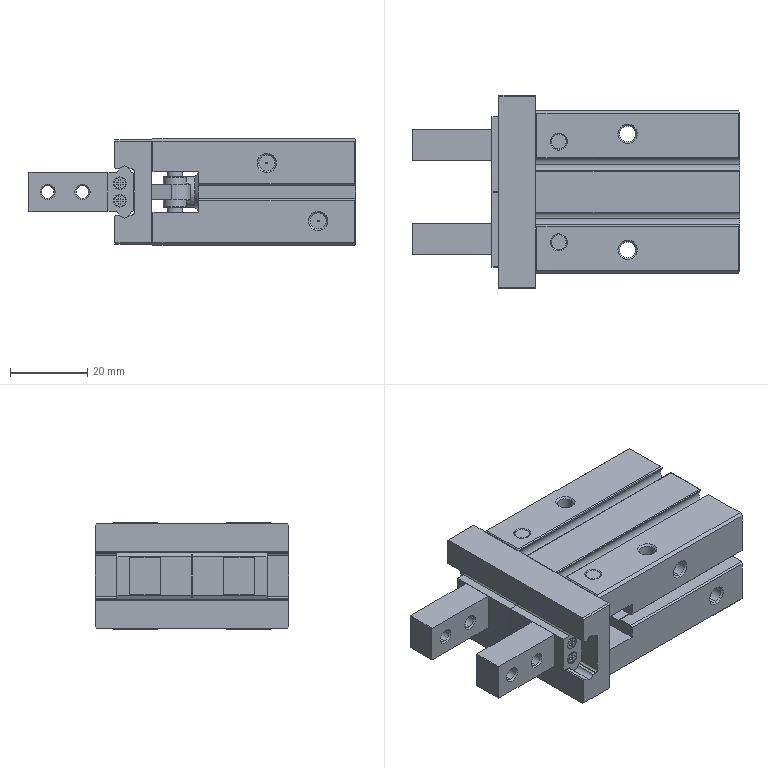Part | STEP file | HFZ20_CL_ | 3 solids | 459 faces | box 84.7 x 50 x 27.6 mm | volume 63972 mm3 | plane 240 | cylinder 144 | cone 67 | torus 8 | commonest cylinder face diameters 4.134 x20 0.4 x16 0.8 x10 3 x10 4 x10 2.5 x9